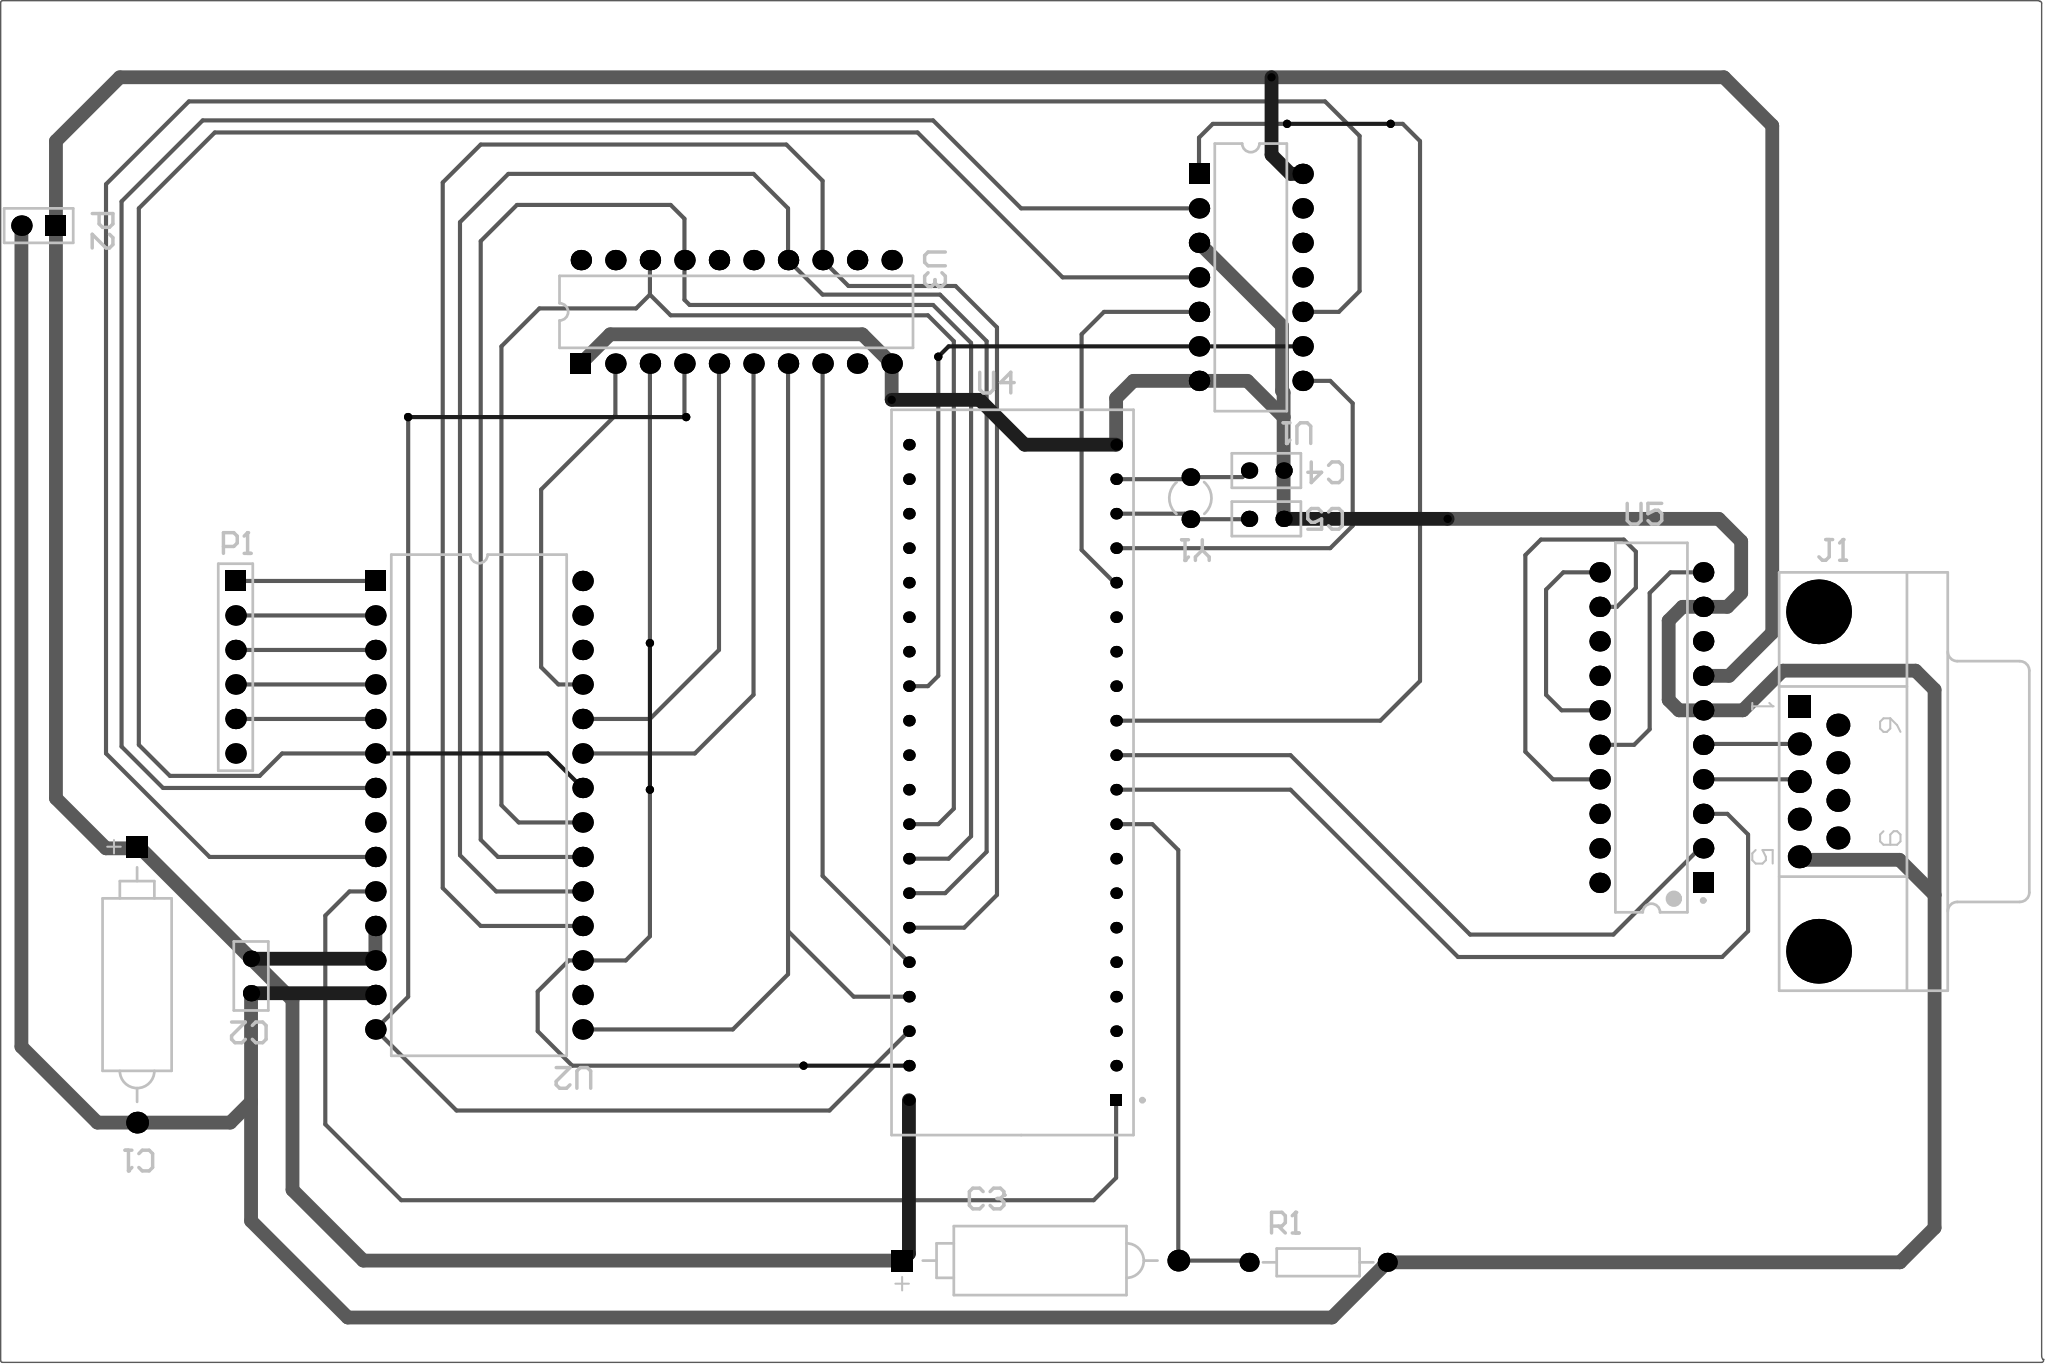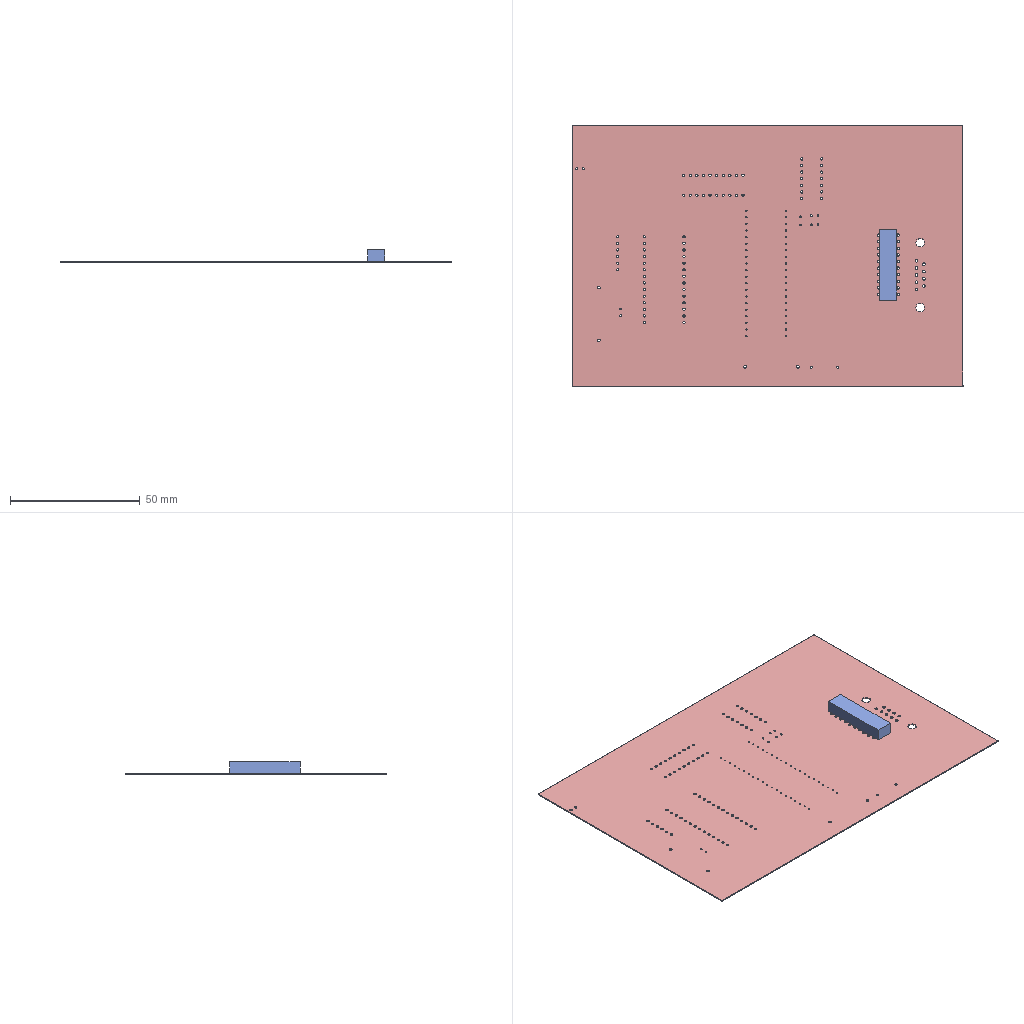Circuit board layout | Altium Designer | box 150.3 x 100.3 x 5 mm
Layer stack:
# Altium Designer layer stack of  (unit mm; dielectric type: 0 none, 1 core, 2 prepreg, 3 surface material)
index,name,kind,layer,copper_thickness_mm,dielectric_type,dielectric_thickness_mm,dielectric_material,dielectric_constant
0,Top Paste,other,,,,,,
1,Top Overlay,other,,,,,,
2,Top Solder,dielectric,,,3,0.0102,Solder Resist,3.5
3,Top Layer,copper,Top Layer,0.0356,,,,
4,Dielectric 1,dielectric,,,0,0.32,FR-4,4.8
5,Bottom Layer,copper,Bottom Layer,0.0356,,,,
6,Bottom Solder,dielectric,,,3,0.0102,Solder Resist,3.5
7,Bottom Overlay,other,,,,,,
8,Bottom Paste,other,,,,,,
# drill layer pairs: low layer,high layer
drill_pair,Top Layer,Bottom Layer
Part placement:
Designator,Comment,Layer,Footprint,Center-X(mm),Center-Y(mm),Rotation
Y1,XTAL,TopLayer,R38,112.776,88.9,180
U5,MAX233AEPP,TopLayer,PP20,146.685,72.009,180
U4,DS5000T-32-16,TopLayer,ENDIP40A,99.695,68.707,90
U3,DM54S373J,TopLayer,J20A,79.375,102.616,360
U2,ADC0809CCN,TopLayer,N28B,60.452,66.294,270
U1,SN74LS02N,TopLayer,N014,117.221,105.156,270
R1,10K,TopLayer,AXIAL-0.4,122.174,32.639,180
P2,Header 2,TopLayer,HDR1X2,28.067,108.966,180
P1,Header 6,TopLayer,HDR1X6,42.545,76.454,270
J1,D Connector 9,TopLayer,DSUB1.385-2H9,158.981,68.036,270
C5,104,TopLayer,RAD-0.1,118.364,87.376,360
C4,104,TopLayer,RAD-0.1,118.364,90.932,180
C3,10UF,TopLayer,POLAR0.8,101.727,32.766,180
C2,104,TopLayer,RAD-0.1,43.688,53.721,270
C1,10UF,TopLayer,POLAR0.8,35.306,53.086,90
Pad and via stacks:
# Altium Designer via and pad stacks of  (unit mm). Each distinct definition once, with the count of objects using it.
# via: kind,start_layer,end_layer,hole_mm,diameter_mm,mode(0 simple;1 top-mid-bottom;2 full stack),diameter_per_layer,count,example_net
# pad: kind,layer,hole_mm,hole_type(0 round;1 square;2 slot),plating,top_size,top_shape(1 round;2 rect;3 octagon;9 rounded rect),mid_size,bottom_size,mode,footprint,size_per_layer,count,example
pad,Multi-Layer,0.9,0,plated,1.5x1.5,1,1.5x1.5,1.5x1.5,0,N28B,,27,U2.16
pad,Multi-Layer,0.9,0,plated,1.5x1.5,1,1.5x1.5,1.5x1.5,0,N014,,13,U1.8
pad,Multi-Layer,0.9,0,plated,1.5x1.5,2,1.5x1.5,1.5x1.5,0,N014,,1,U1.1
pad,Multi-Layer,0.7,0,plated,1.2x1.2,1,1.2x1.2,1.2x1.2,0,RAD-0.1,,6,C2.1
pad,Multi-Layer,1,0,plated,1.6x1.6,1,1.6x1.6,1.6x1.6,0,POLAR0.8,,2,C1.2
pad,Multi-Layer,1,0,plated,1.6x1.6,2,1.6x1.6,1.6x1.6,0,POLAR0.8,,2,C1.1
pad,Multi-Layer,0.9,0,plated,1.5x1.5,2,1.5x1.5,1.5x1.5,0,N28B,,1,U2.1
pad,Multi-Layer,0.9,0,plated,1.5x1.5,1,1.5x1.5,1.5x1.5,0,J20A,,19,U3.11
pad,Multi-Layer,0.9,0,plated,1.5x1.5,2,1.5x1.5,1.5x1.5,0,J20A,,1,U3.1
pad,Multi-Layer,0.9,0,plated,1.5x1.5,2,1.5x1.5,1.5x1.5,0,HDR1X6,,1,P1.1
pad,Multi-Layer,0.9,0,plated,1.5x1.5,1,1.5x1.5,1.5x1.5,0,HDR1X6,,5,P1.2
pad,Multi-Layer,0.5,0,plated,0.85x0.85,1,0.85x0.85,0.85x0.85,0,ENDIP40A,,39,U4.9
pad,Multi-Layer,0.5,0,plated,0.85x0.85,2,0.85x0.85,0.85x0.85,0,ENDIP40A,,1,U4.1
pad,Multi-Layer,0.9,0,plated,1.5x1.5,2,1.5x1.5,1.5x1.5,0,PP20,,1,U5.1
pad,Multi-Layer,0.9,0,plated,1.5x1.5,1,1.5x1.5,1.5x1.5,0,PP20,,19,U5.2
pad,Multi-Layer,3.26,0,plated,4.76x4.76,1,4.76x4.76,4.76x4.76,0,DSUB1.385-2H9,,2,J1.11
pad,Multi-Layer,1.09,0,plated,1.69x1.69,2,1.69x1.69,1.69x1.69,0,DSUB1.385-2H9,,1,J1.1
pad,Multi-Layer,1.09,0,plated,1.69x1.69,1,1.69x1.69,1.69x1.69,0,DSUB1.385-2H9,,8,J1.6
pad,Multi-Layer,0.85,0,plated,1.4x1.4,1,1.4x1.4,1.4x1.4,0,AXIAL-0.4,,2,R1.1
pad,Multi-Layer,0.7,0,plated,1.3x1.3,1,1.3x1.3,1.3x1.3,0,R38,,2,Y1.1
pad,Multi-Layer,0.9,0,plated,1.5x1.5,2,1.5x1.5,1.5x1.5,0,HDR1X2,,1,P2.1
pad,Multi-Layer,0.9,0,plated,1.5x1.5,1,1.5x1.5,1.5x1.5,0,HDR1X2,,1,P2.2
via,Top Layer,Bottom Layer,0.3048,0.6096,0,,11,GND
Design rules, without the lines most boards share:
# Altium Designer design rules of  (exported by Altium Designer, unit mm)
# columns: name | kind | enabled | priority | scope1 | scope2 | descriptor | typed fields (field=value)
SilkToSilkClearance | 55 | enabled | 1 | All | All | Silk to Silk (Clearance=0mil) (All),(All) |
SilkToSolderMaskClearance | 54 | enabled | 1 | IsPad | All | Silk To Solder Mask (Clearance=0mil) (IsPad),(All) |
MinimumSolderMaskSliver | 53 | enabled | 1 | All | All | Minimum Solder Mask Sliver (Gap=0mil) (All),(All) |
HoleToHoleClearance | 52 | enabled | 1 | All | All | Hole To Hole Clearance (Gap=10mil) (All),(All) | gap=0.254
DiffPairsRouting | 51 | enabled | 1 | All | All | Differential Pairs Uncoupled Length using the Gap Constraints (Min=10mil) (Max=10mil) (Prefered=10mil)  and Width Constraints (Min=15mil) (Max=15mil) (Prefered=15mil) (All) |
HoleSize | 42 | enabled | 1 | All | All | Hole Size Constraint (Min=1mil) (Max=3937.008mil) (All) |
SolderMaskExpansion | 13 | enabled | 1 | All | All | Solder Mask Expansion (Expansion =4mil) (All) | expansion=0.1016
PasteMaskExpansion | 14 | enabled | 1 | All | All | Paste Mask Expansion (Expansion =0mil) (All) | expansion=0
RoutingVias | 11 | enabled | 1 | All | All | Routing Via (MinHoleWidth=28mil) (MaxHoleWidth=28mil) (PreferredHoleWidth=28mil) (MinWidth=50mil) (MaxWidth=50mil) (PreferedWidth=50mil) (All) | via_min_hole=0.7112 via_max_hole=0.7112 via_preferred_diameter=1.27 via_preferred_hole=0.7112
Width | 2 | enabled | 1 | All | All | Width Constraint (Min=12mil) (Max=40mil) (Preferred=20mil) (All) |
PolygonConnect | 20 | enabled | 1 | All | All | Polygon Connect Rule(Relief Connect )(Conductor Width=10mil) (Relief Angle=90 Angle) (Entries=4) (Air Gap Width=10mil) (All),(All) | connect_style(0=relief,1=direct,2=none)=0 relief_conductor_width=0.254 relief_entries=4
PlaneConnect | 6 | enabled | 1 | All | All | Power Plane Connect Rule(Relief Connect )(Expansion=20mil) (Conductor Width=10mil) (Air Gap=10mil) (Entries=4) (All) | relief_conductor_width=0.254 relief_entries=4 relief_expansion=0.508
Clearance | 0 | enabled | 1 | All | All | Clearance Constraint (Gap=10mil) (All),(All) | gap=0.254
Classes set for this board:
# Altium Designer classes of  (member kind: 0 net, 1 component, 2 from-to, 3 pad, 4 layer, 5 differential pair, 6 design channel, 7 polygon, 8 structure, 9 xSignal)
# columns: class name | member kind | superclass | members
Sheet1 | 1 | no | C1; C2; C3; C4; C5; J1; P1; P2; R1; U1; U2; U3; U4; U5; Y1;